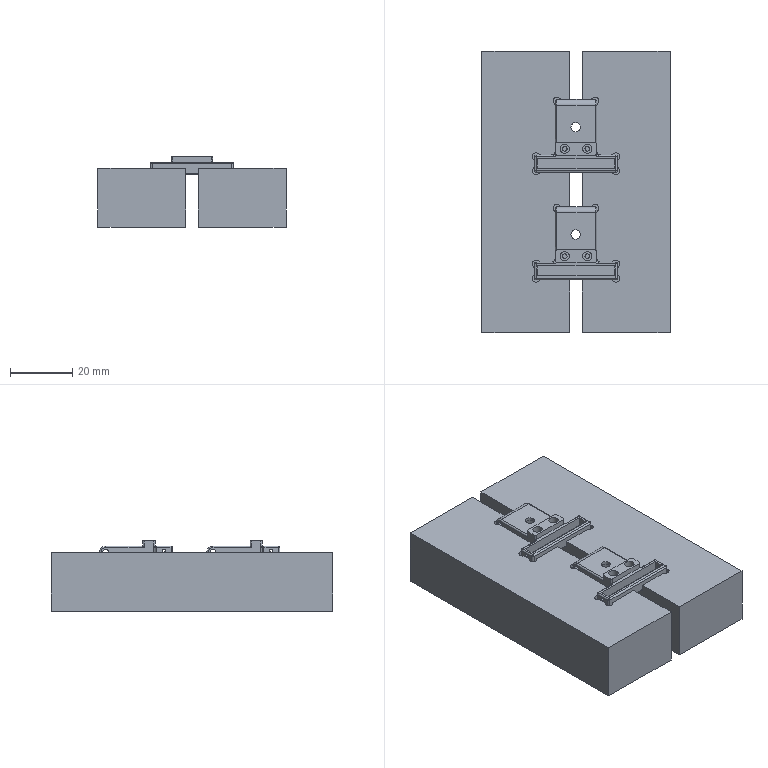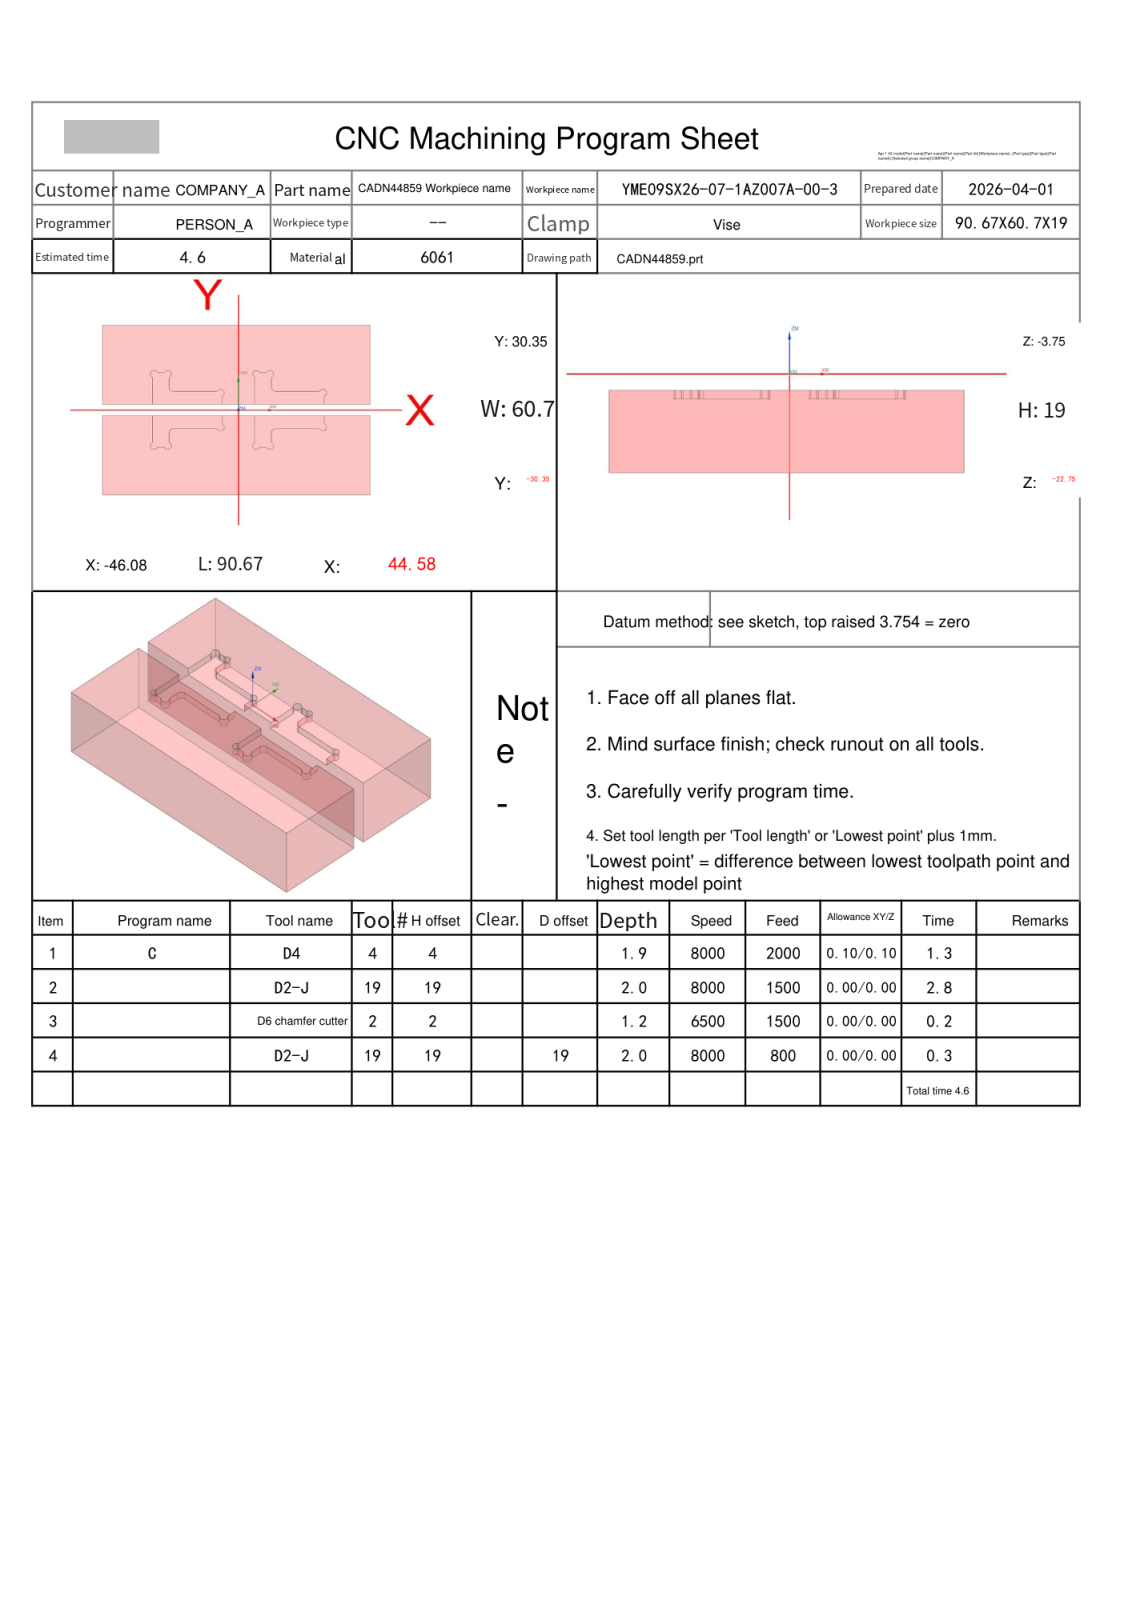NC program | NX | posted by the shop | part box 60.696 x 90.669 x 22.754 mm
Lines 950 to 1992 of 8014:
N2 T19 M06
(D2-J  D=2. R=0. H=19 ce=0.00 di=0.00)
G00 G90 G54 X27.884 Y3.83 M03 S8000
G43 H19 Z46.246
M08
Z-3.654
G01 X27.887 Z-3.684 F800.
X27.894 Y3.832 Z-3.712
X27.905 Y3.835 Z-3.736
X27.92 Y3.84 Z-3.758
X27.936 Y3.846 Z-3.777
X27.955 Y3.854 Z-3.794
X27.975 Y3.864 Z-3.808
X27.994 Y3.876 Z-3.82
X28.014 Y3.89 Z-3.83
X28.033 Y3.907 Z-3.838
X28.049 Y3.926 Z-3.844
X28.064 Y3.947 Z-3.849
X28.075 Y3.972 Z-3.852
X28.082 Y3.999 Z-3.853
X28.084 Y4.03 Z-3.854
Y4.698
G02 X28.727 Y5.929 I1.5 J0.0
G03 X28.834 Y6.134 I-.143 J.205
X28.584 Y6.384 I-.25 J0.0
X28.379 Y6.277 I0.0 J-.25
G02 X27.148 Y5.634 I-1.231 J.857
G01 X26.48
X26.454 Y5.62 Z-3.855
X26.45 Y5.582 Z-3.856
X26.465 Y5.524 Z-3.859
X26.497 Y5.448 Z-3.862
X26.544 Y5.359 Z-3.866
X26.602 Y5.26 Z-3.871
X26.671 Y5.156 Z-3.876
X26.747 Y5.049 Z-3.881
X26.974 Y4.772 Z-3.896
X27.229 Y4.516 Z-3.912
X27.504 Y4.289 Z-3.927
X27.61 Y4.214 Z-3.932
X27.714 Y4.146 Z-3.937
X27.811 Y4.089 Z-3.942
X27.9 Y4.043 Z-3.946
X27.975 Y4.013 Z-3.949
X28.033 Y3.999 Z-3.952
X28.071 Y4.003 Z-3.953
X28.084 Y4.03 Z-3.954
Y4.698
G02 X28.727 Y5.929 I1.5 J0.0
G03 X28.834 Y6.134 I-.143 J.205
X28.584 Y6.384 I-.25 J0.0
X28.379 Y6.277 I0.0 J-.25
G02 X27.148 Y5.634 I-1.231 J.857
G01 X26.48
X26.454 Y5.62 Z-3.955
X26.45 Y5.582 Z-3.956
X26.465 Y5.524 Z-3.959
X26.497 Y5.448 Z-3.962
X26.544 Y5.359 Z-3.966
X26.602 Y5.26 Z-3.971
X26.671 Y5.156 Z-3.976
X26.747 Y5.049 Z-3.981
X26.974 Y4.772 Z-3.996
X27.229 Y4.516 Z-4.012
X27.504 Y4.289 Z-4.027
X27.61 Y4.214 Z-4.032
X27.714 Y4.146 Z-4.037
X27.811 Y4.089 Z-4.042
X27.9 Y4.043 Z-4.046
X27.975 Y4.013 Z-4.049
X28.033 Y3.999 Z-4.052
X28.071 Y4.003 Z-4.053
X28.084 Y4.03 Z-4.054
Y4.698
G02 X28.727 Y5.929 I1.5 J0.0
G03 X28.834 Y6.134 I-.143 J.205
X28.584 Y6.384 I-.25 J0.0
X28.379 Y6.277 I0.0 J-.25
G02 X27.148 Y5.634 I-1.231 J.857
G01 X26.48
X26.454 Y5.62 Z-4.055
X26.45 Y5.582 Z-4.056
X26.465 Y5.524 Z-4.059
X26.497 Y5.448 Z-4.062
X26.544 Y5.359 Z-4.066
X26.602 Y5.26 Z-4.071
X26.671 Y5.156 Z-4.076
X26.747 Y5.049 Z-4.081
X26.974 Y4.772 Z-4.096
X27.229 Y4.516 Z-4.112
X27.504 Y4.289 Z-4.127
X27.61 Y4.214 Z-4.132
X27.714 Y4.146 Z-4.137
X27.811 Y4.089 Z-4.142
X27.9 Y4.043 Z-4.146
X27.975 Y4.013 Z-4.149
X28.033 Y3.999 Z-4.152
X28.071 Y4.003 Z-4.153
X28.084 Y4.03 Z-4.154
Y4.698
G02 X28.727 Y5.929 I1.5 J0.0
G03 X28.834 Y6.134 I-.143 J.205
X28.584 Y6.384 I-.25 J0.0
X28.379 Y6.277 I0.0 J-.25
G02 X27.148 Y5.634 I-1.231 J.857
G01 X26.48
X26.454 Y5.62 Z-4.155
X26.45 Y5.582 Z-4.156
X26.465 Y5.524 Z-4.159
X26.497 Y5.448 Z-4.162
X26.544 Y5.359 Z-4.166
X26.602 Y5.26 Z-4.171
X26.671 Y5.156 Z-4.176
X26.747 Y5.049 Z-4.181
X26.974 Y4.772 Z-4.196
X27.229 Y4.516 Z-4.212
X27.504 Y4.289 Z-4.227
X27.61 Y4.214 Z-4.232
X27.714 Y4.146 Z-4.237
X27.811 Y4.089 Z-4.242
X27.9 Y4.043 Z-4.246
X27.975 Y4.013 Z-4.249
X28.033 Y3.999 Z-4.252
X28.071 Y4.003 Z-4.253
X28.084 Y4.03 Z-4.254
Y4.698
G02 X28.727 Y5.929 I1.5 J0.0
G03 X28.834 Y6.134 I-.143 J.205
X28.584 Y6.384 I-.25 J0.0
X28.379 Y6.277 I0.0 J-.25
G02 X27.148 Y5.634 I-1.231 J.857
G01 X26.48
X26.454 Y5.62 Z-4.255
X26.45 Y5.582 Z-4.256
X26.465 Y5.524 Z-4.259
X26.497 Y5.448 Z-4.262
X26.544 Y5.359 Z-4.266
X26.602 Y5.26 Z-4.271
X26.671 Y5.156 Z-4.276
X26.747 Y5.049 Z-4.281
X26.974 Y4.772 Z-4.296
X27.229 Y4.516 Z-4.312
X27.504 Y4.289 Z-4.327
X27.61 Y4.214 Z-4.332
X27.714 Y4.146 Z-4.337
X27.811 Y4.089 Z-4.342
X27.9 Y4.043 Z-4.346
X27.975 Y4.013 Z-4.349
X28.033 Y3.999 Z-4.352
X28.071 Y4.003 Z-4.353
X28.084 Y4.03 Z-4.354
Y4.698
G02 X28.727 Y5.929 I1.5 J0.0
G03 X28.834 Y6.134 I-.143 J.205
X28.584 Y6.384 I-.25 J0.0
X28.379 Y6.277 I0.0 J-.25
G02 X27.148 Y5.634 I-1.231 J.857
G01 X26.48
X26.454 Y5.62 Z-4.355
X26.45 Y5.582 Z-4.356
X26.465 Y5.524 Z-4.359
X26.497 Y5.448 Z-4.362
X26.544 Y5.359 Z-4.366
X26.602 Y5.26 Z-4.371
X26.671 Y5.156 Z-4.376
X26.747 Y5.049 Z-4.381
X26.974 Y4.772 Z-4.396
X27.229 Y4.516 Z-4.412
X27.504 Y4.289 Z-4.427
X27.61 Y4.214 Z-4.432
X27.714 Y4.146 Z-4.437
X27.811 Y4.089 Z-4.442
X27.9 Y4.043 Z-4.446
X27.975 Y4.013 Z-4.449
X28.033 Y3.999 Z-4.452
X28.071 Y4.003 Z-4.453
X28.084 Y4.03 Z-4.454
Y4.698
G02 X28.727 Y5.929 I1.5 J0.0
G03 X28.834 Y6.134 I-.143 J.205
X28.584 Y6.384 I-.25 J0.0
X28.379 Y6.277 I0.0 J-.25
G02 X27.148 Y5.634 I-1.231 J.857
G01 X26.48
X26.454 Y5.62 Z-4.455
X26.45 Y5.582 Z-4.456
X26.465 Y5.524 Z-4.459
X26.497 Y5.448 Z-4.462
X26.544 Y5.359 Z-4.466
X26.602 Y5.26 Z-4.471
X26.671 Y5.156 Z-4.476
X26.747 Y5.049 Z-4.481
X26.974 Y4.772 Z-4.496
X27.229 Y4.516 Z-4.512
X27.504 Y4.289 Z-4.527
X27.61 Y4.214 Z-4.532
X27.714 Y4.146 Z-4.537
X27.811 Y4.089 Z-4.542
X27.9 Y4.043 Z-4.546
X27.975 Y4.013 Z-4.549
X28.033 Y3.999 Z-4.552
X28.071 Y4.003 Z-4.553
X28.084 Y4.03 Z-4.554
Y4.698
G02 X28.727 Y5.929 I1.5 J0.0
G03 X28.834 Y6.134 I-.143 J.205
X28.584 Y6.384 I-.25 J0.0
X28.379 Y6.277 I0.0 J-.25
G02 X27.148 Y5.634 I-1.231 J.857
G01 X26.48
X26.454 Y5.62 Z-4.555
X26.45 Y5.582 Z-4.556
X26.465 Y5.524 Z-4.559
X26.497 Y5.448 Z-4.562
X26.544 Y5.359 Z-4.566
X26.602 Y5.26 Z-4.571
X26.671 Y5.156 Z-4.576
X26.747 Y5.049 Z-4.581
X26.974 Y4.772 Z-4.596
X27.229 Y4.516 Z-4.612
X27.504 Y4.289 Z-4.627
X27.61 Y4.214 Z-4.632
X27.714 Y4.146 Z-4.637
X27.811 Y4.089 Z-4.642
X27.9 Y4.043 Z-4.646
X27.975 Y4.013 Z-4.649
X28.033 Y3.999 Z-4.652
X28.071 Y4.003 Z-4.653
X28.084 Y4.03 Z-4.654
Y4.698
G02 X28.727 Y5.929 I1.5 J0.0
G03 X28.834 Y6.134 I-.143 J.205
X28.584 Y6.384 I-.25 J0.0
X28.379 Y6.277 I0.0 J-.25
G02 X27.148 Y5.634 I-1.231 J.857
G01 X26.48
X26.454 Y5.62 Z-4.655
X26.45 Y5.582 Z-4.656
X26.465 Y5.524 Z-4.659
X26.497 Y5.448 Z-4.662
X26.544 Y5.359 Z-4.666
X26.602 Y5.26 Z-4.671
X26.671 Y5.156 Z-4.676
X26.747 Y5.049 Z-4.681
X26.974 Y4.772 Z-4.696
X27.229 Y4.516 Z-4.712
X27.504 Y4.289 Z-4.727
X27.61 Y4.214 Z-4.732
X27.714 Y4.146 Z-4.737
X27.811 Y4.089 Z-4.742
X27.9 Y4.043 Z-4.746
X27.975 Y4.013 Z-4.749
X28.033 Y3.999 Z-4.752
X28.071 Y4.003 Z-4.753
X28.084 Y4.03 Z-4.754
Y4.698
G02 X28.727 Y5.929 I1.5 J0.0
G03 X28.834 Y6.134 I-.143 J.205
X28.584 Y6.384 I-.25 J0.0
X28.379 Y6.277 I0.0 J-.25
G02 X27.148 Y5.634 I-1.231 J.857
G01 X26.48
X26.454 Y5.62 Z-4.755
X26.45 Y5.582 Z-4.756
X26.465 Y5.524 Z-4.759
X26.497 Y5.448 Z-4.762
X26.544 Y5.359 Z-4.766
X26.602 Y5.26 Z-4.771
X26.671 Y5.156 Z-4.776
X26.747 Y5.049 Z-4.781
X26.974 Y4.772 Z-4.796
X27.229 Y4.516 Z-4.812
X27.504 Y4.289 Z-4.827
X27.61 Y4.214 Z-4.832
X27.714 Y4.146 Z-4.837
X27.811 Y4.089 Z-4.842
X27.9 Y4.043 Z-4.846
X27.975 Y4.013 Z-4.849
X28.033 Y3.999 Z-4.852
X28.071 Y4.003 Z-4.853
X28.084 Y4.03 Z-4.854
Y4.698
G02 X28.727 Y5.929 I1.5 J0.0
G03 X28.834 Y6.134 I-.143 J.205
X28.584 Y6.384 I-.25 J0.0
X28.379 Y6.277 I0.0 J-.25
G02 X27.148 Y5.634 I-1.231 J.857
G01 X26.48
X26.454 Y5.62 Z-4.855
X26.45 Y5.582 Z-4.856
X26.465 Y5.524 Z-4.859
X26.497 Y5.448 Z-4.862
X26.544 Y5.359 Z-4.866
X26.602 Y5.26 Z-4.871
X26.671 Y5.156 Z-4.876
X26.747 Y5.049 Z-4.881
X26.974 Y4.772 Z-4.896
X27.229 Y4.516 Z-4.912
X27.504 Y4.289 Z-4.927
X27.61 Y4.214 Z-4.932
X27.714 Y4.146 Z-4.937
X27.811 Y4.089 Z-4.942
X27.9 Y4.043 Z-4.946
X27.975 Y4.013 Z-4.949
X28.033 Y3.999 Z-4.952
X28.071 Y4.003 Z-4.953
X28.084 Y4.03 Z-4.954
Y4.698
G02 X28.727 Y5.929 I1.5 J0.0
G03 X28.834 Y6.134 I-.143 J.205
X28.584 Y6.384 I-.25 J0.0
X28.379 Y6.277 I0.0 J-.25
G02 X27.148 Y5.634 I-1.231 J.857
G01 X26.48
X26.454 Y5.62 Z-4.955
X26.45 Y5.582 Z-4.956
X26.465 Y5.524 Z-4.959
X26.497 Y5.448 Z-4.962
X26.544 Y5.359 Z-4.966
X26.602 Y5.26 Z-4.971
X26.671 Y5.156 Z-4.976
X26.747 Y5.049 Z-4.981
X26.974 Y4.772 Z-4.996
X27.229 Y4.516 Z-5.012
X27.504 Y4.289 Z-5.027
X27.61 Y4.214 Z-5.032
X27.714 Y4.146 Z-5.037
X27.811 Y4.089 Z-5.042
X27.9 Y4.043 Z-5.046
X27.975 Y4.013 Z-5.049
X28.033 Y3.999 Z-5.052
X28.071 Y4.003 Z-5.053
X28.084 Y4.03 Z-5.054
Y4.698
G02 X28.727 Y5.929 I1.5 J0.0
G03 X28.834 Y6.134 I-.143 J.205
X28.584 Y6.384 I-.25 J0.0
X28.379 Y6.277 I0.0 J-.25
G02 X27.148 Y5.634 I-1.231 J.857
G01 X26.48
X26.454 Y5.62 Z-5.055
X26.45 Y5.582 Z-5.056
X26.465 Y5.524 Z-5.059
X26.497 Y5.448 Z-5.062
X26.544 Y5.359 Z-5.066
X26.602 Y5.26 Z-5.071
X26.671 Y5.156 Z-5.076
X26.747 Y5.049 Z-5.081
X26.974 Y4.772 Z-5.096
X27.229 Y4.516 Z-5.112
X27.504 Y4.289 Z-5.127
X27.61 Y4.214 Z-5.132
X27.714 Y4.146 Z-5.137
X27.811 Y4.089 Z-5.142
X27.9 Y4.043 Z-5.146
X27.975 Y4.013 Z-5.149
X28.033 Y3.999 Z-5.152
X28.071 Y4.003 Z-5.153
X28.084 Y4.03 Z-5.154
Y4.698
G02 X28.727 Y5.929 I1.5 J0.0
G03 X28.834 Y6.134 I-.143 J.205
X28.584 Y6.384 I-.25 J0.0
X28.379 Y6.277 I0.0 J-.25
G02 X27.148 Y5.634 I-1.231 J.857
G01 X26.48
X26.454 Y5.62 Z-5.155
X26.45 Y5.582 Z-5.156
X26.465 Y5.524 Z-5.159
X26.497 Y5.448 Z-5.162
X26.544 Y5.359 Z-5.166
X26.602 Y5.26 Z-5.171
X26.671 Y5.156 Z-5.176
X26.747 Y5.049 Z-5.181
X26.974 Y4.772 Z-5.196
X27.229 Y4.516 Z-5.212
X27.504 Y4.289 Z-5.227
X27.61 Y4.214 Z-5.232
X27.714 Y4.146 Z-5.237
X27.811 Y4.089 Z-5.242
X27.9 Y4.043 Z-5.246
X27.975 Y4.013 Z-5.249
X28.033 Y3.999 Z-5.252
X28.071 Y4.003 Z-5.253
X28.084 Y4.03 Z-5.254
Y4.698
G02 X28.727 Y5.929 I1.5 J0.0
G03 X28.834 Y6.134 I-.143 J.205
X28.584 Y6.384 I-.25 J0.0
X28.379 Y6.277 I0.0 J-.25
G02 X27.148 Y5.634 I-1.231 J.857
G01 X26.48
X26.454 Y5.62 Z-5.255
X26.45 Y5.582 Z-5.256
X26.465 Y5.524 Z-5.259
X26.497 Y5.448 Z-5.262
X26.544 Y5.359 Z-5.266
X26.602 Y5.26 Z-5.271
X26.671 Y5.156 Z-5.276
X26.747 Y5.049 Z-5.281
X26.974 Y4.772 Z-5.296
X27.229 Y4.516 Z-5.312
X27.504 Y4.289 Z-5.327
X27.61 Y4.214 Z-5.332
X27.714 Y4.146 Z-5.337
X27.811 Y4.089 Z-5.342
X27.9 Y4.043 Z-5.346
X27.975 Y4.013 Z-5.349
X28.033 Y3.999 Z-5.352
X28.071 Y4.003 Z-5.353
X28.084 Y4.03 Z-5.354
Y4.698
G02 X28.727 Y5.929 I1.5 J0.0
G03 X28.834 Y6.134 I-.143 J.205
X28.584 Y6.384 I-.25 J0.0
X28.379 Y6.277 I0.0 J-.25
G02 X27.148 Y5.634 I-1.231 J.857
G01 X26.48
X26.454 Y5.62 Z-5.355
X26.45 Y5.582 Z-5.356
X26.465 Y5.524 Z-5.359
X26.497 Y5.448 Z-5.362
X26.544 Y5.359 Z-5.366
X26.602 Y5.26 Z-5.371
X26.671 Y5.156 Z-5.376
X26.747 Y5.049 Z-5.381
X26.974 Y4.772 Z-5.396
X27.229 Y4.516 Z-5.412
X27.504 Y4.289 Z-5.427
X27.61 Y4.214 Z-5.432
X27.714 Y4.146 Z-5.437
X27.811 Y4.089 Z-5.442
X27.9 Y4.043 Z-5.446
X27.975 Y4.013 Z-5.449
X28.033 Y3.999 Z-5.452
X28.071 Y4.003 Z-5.453
X28.084 Y4.03 Z-5.454
Y4.698
G02 X28.727 Y5.929 I1.5 J0.0
G03 X28.834 Y6.134 I-.143 J.205
X28.584 Y6.384 I-.25 J0.0
X28.379 Y6.277 I0.0 J-.25
G02 X27.148 Y5.634 I-1.231 J.857
G01 X26.48
X26.454 Y5.62 Z-5.455
X26.45 Y5.582 Z-5.456
X26.465 Y5.524 Z-5.459
X26.497 Y5.448 Z-5.462
X26.544 Y5.359 Z-5.466
X26.602 Y5.26 Z-5.471
X26.671 Y5.156 Z-5.476
X26.747 Y5.049 Z-5.481
X26.974 Y4.772 Z-5.496
X27.229 Y4.516 Z-5.512
X27.504 Y4.289 Z-5.527
X27.61 Y4.214 Z-5.532
X27.714 Y4.146 Z-5.537
X27.811 Y4.089 Z-5.542
X27.9 Y4.043 Z-5.546
X27.975 Y4.013 Z-5.549
X28.033 Y3.999 Z-5.552
X28.071 Y4.003 Z-5.553
X28.084 Y4.03 Z-5.554
Y4.698
G02 X28.727 Y5.929 I1.5 J0.0
G03 X28.834 Y6.134 I-.143 J.205
X28.584 Y6.384 I-.25 J0.0
X28.379 Y6.277 I0.0 J-.25
G02 X27.148 Y5.634 I-1.231 J.857
G01 X26.48
X26.454 Y5.62 Z-5.555
X26.45 Y5.582 Z-5.556
X26.465 Y5.524 Z-5.559
X26.497 Y5.448 Z-5.562
X26.544 Y5.359 Z-5.566
X26.602 Y5.26 Z-5.571
X26.671 Y5.156 Z-5.576
X26.747 Y5.049 Z-5.581
X26.974 Y4.772 Z-5.596
X27.229 Y4.516 Z-5.612
X27.504 Y4.289 Z-5.627
X27.61 Y4.214 Z-5.632
X27.714 Y4.146 Z-5.637
X27.811 Y4.089 Z-5.642
X27.9 Y4.043 Z-5.646
X27.975 Y4.013 Z-5.649
X28.033 Y3.999 Z-5.652
X28.071 Y4.003 Z-5.653
X28.084 Y4.03 Z-5.654
Y4.698
G02 X28.727 Y5.929 I1.5 J0.0
G03 X28.834 Y6.134 I-.143 J.205
X28.584 Y6.384 I-.25 J0.0
X28.379 Y6.277 I0.0 J-.25
G02 X27.148 Y5.634 I-1.231 J.857
G01 X26.48
X26.454 Y5.62 Z-5.655
X26.45 Y5.582 Z-5.656
X26.465 Y5.524 Z-5.659
X26.497 Y5.448 Z-5.662
X26.544 Y5.359 Z-5.666
X26.602 Y5.26 Z-5.671
X26.671 Y5.156 Z-5.676
X26.747 Y5.049 Z-5.681
X26.974 Y4.772 Z-5.696
X27.229 Y4.516 Z-5.712
X27.504 Y4.289 Z-5.727
X27.61 Y4.214 Z-5.732
X27.714 Y4.146 Z-5.737
X27.811 Y4.089 Z-5.742
X27.9 Y4.043 Z-5.746
X27.975 Y4.013 Z-5.749
X28.033 Y3.999 Z-5.752
X28.071 Y4.003 Z-5.753
X28.084 Y4.03 Z-5.754
Y4.698
G02 X28.727 Y5.929 I1.5 J0.0
G03 X28.834 Y6.134 I-.143 J.205
X28.584 Y6.384 I-.25 J0.0
X28.379 Y6.277 I0.0 J-.25
G02 X27.148 Y5.634 I-1.231 J.857
G01 X26.48
X26.45 Y5.631 Z-5.753
X26.423 Y5.624 Z-5.752
X26.4 Y5.613 Z-5.749
X26.379 Y5.599 Z-5.744
X26.361 Y5.582 Z-5.738
X26.346 Y5.563 Z-5.73
X26.333 Y5.544 Z-5.72
X26.323 Y5.524 Z-5.708
X26.314 Y5.504 Z-5.694
X26.307 Y5.486 Z-5.677
X26.302 Y5.469 Z-5.658
X26.299 Y5.455 Z-5.636
X26.296 Y5.443 Z-5.612
X26.295 Y5.436 Z-5.584
Y5.434 Z-5.554
G00 Z46.246
X9.945 Y10.544
Z-3.654
G01 X9.947 Z-3.684
X9.955 Y10.546 Z-3.712
X9.966 Y10.549 Z-3.736
X9.98 Y10.554 Z-3.758
X9.997 Y10.56 Z-3.777
X10.016 Y10.568 Z-3.794
X10.036 Y10.578 Z-3.808
X10.056 Y10.59 Z-3.82
X10.076 Y10.604 Z-3.83
X10.095 Y10.621 Z-3.838
X10.112 Y10.64 Z-3.844
X10.127 Y10.662 Z-3.849
X10.138 Y10.686 Z-3.852
X10.145 Y10.713 Z-3.853
X10.148 Y10.744 Z-3.854
Y11.412
G02 X10.791 Y12.643 I1.5 J0.0
G03 X10.898 Y12.848 I-.143 J.205
X10.648 Y13.098 I-.25 J0.0
X10.443 Y12.991 I0.0 J-.25
G02 X9.212 Y12.348 I-1.231 J.857
G01 X8.543
X8.517 Y12.335 Z-3.855
X8.512 Y12.297 Z-3.856
X8.526 Y12.238 Z-3.859
X8.557 Y12.162 Z-3.862
X8.602 Y12.073 Z-3.866
X8.66 Y11.975 Z-3.871
X8.727 Y11.87 Z-3.876
X8.802 Y11.763 Z-3.881
X9.029 Y11.487 Z-3.896
X9.285 Y11.23 Z-3.912
X9.562 Y11.003 Z-3.927
X9.669 Y10.928 Z-3.932
X9.773 Y10.86 Z-3.937
X9.872 Y10.803 Z-3.942
X9.961 Y10.758 Z-3.946
X10.037 Y10.727 Z-3.949
X10.096 Y10.713 Z-3.952
X10.134 Y10.718 Z-3.953
X10.148 Y10.744 Z-3.954
Y11.412
G02 X10.791 Y12.643 I1.5 J0.0
G03 X10.898 Y12.848 I-.143 J.205
X10.648 Y13.098 I-.25 J0.0
X10.443 Y12.991 I0.0 J-.25
G02 X9.212 Y12.348 I-1.231 J.857
G01 X8.543
X8.517 Y12.335 Z-3.955
X8.512 Y12.297 Z-3.956
X8.526 Y12.238 Z-3.959
X8.557 Y12.162 Z-3.962
X8.602 Y12.073 Z-3.966
X8.66 Y11.975 Z-3.971
X8.727 Y11.87 Z-3.976
X8.802 Y11.763 Z-3.981
X9.029 Y11.487 Z-3.996
X9.285 Y11.23 Z-4.012
X9.562 Y11.003 Z-4.027
X9.669 Y10.928 Z-4.032
X9.773 Y10.86 Z-4.037
X9.872 Y10.803 Z-4.042
X9.961 Y10.758 Z-4.046
X10.037 Y10.727 Z-4.049
X10.096 Y10.713 Z-4.052
X10.134 Y10.718 Z-4.053
X10.148 Y10.744 Z-4.054
Y11.412
G02 X10.791 Y12.643 I1.5 J0.0
G03 X10.898 Y12.848 I-.143 J.205
X10.648 Y13.098 I-.25 J0.0
X10.443 Y12.991 I0.0 J-.25
G02 X9.212 Y12.348 I-1.231 J.857
G01 X8.543
X8.517 Y12.335 Z-4.055
X8.512 Y12.297 Z-4.056
X8.526 Y12.238 Z-4.059
X8.557 Y12.162 Z-4.062
X8.602 Y12.073 Z-4.066
X8.66 Y11.975 Z-4.071
X8.727 Y11.87 Z-4.076
X8.802 Y11.763 Z-4.081
X9.029 Y11.487 Z-4.096
X9.285 Y11.23 Z-4.112
X9.562 Y11.003 Z-4.127
X9.669 Y10.928 Z-4.132
X9.773 Y10.86 Z-4.137
X9.872 Y10.803 Z-4.142
X9.961 Y10.758 Z-4.146
X10.037 Y10.727 Z-4.149
X10.096 Y10.713 Z-4.152
X10.134 Y10.718 Z-4.153
X10.148 Y10.744 Z-4.154
Y11.412
G02 X10.791 Y12.643 I1.5 J0.0
G03 X10.898 Y12.848 I-.143 J.205
X10.648 Y13.098 I-.25 J0.0
X10.443 Y12.991 I0.0 J-.25
G02 X9.212 Y12.348 I-1.231 J.857
G01 X8.543
X8.517 Y12.335 Z-4.155
X8.512 Y12.297 Z-4.156
X8.526 Y12.238 Z-4.159
X8.557 Y12.162 Z-4.162
X8.602 Y12.073 Z-4.166
X8.66 Y11.975 Z-4.171
X8.727 Y11.87 Z-4.176
X8.802 Y11.763 Z-4.181
X9.029 Y11.487 Z-4.196
X9.285 Y11.23 Z-4.212
X9.562 Y11.003 Z-4.227
X9.669 Y10.928 Z-4.232
X9.773 Y10.86 Z-4.237
X9.872 Y10.803 Z-4.242
X9.961 Y10.758 Z-4.246
X10.037 Y10.727 Z-4.249
X10.096 Y10.713 Z-4.252
X10.134 Y10.718 Z-4.253
X10.148 Y10.744 Z-4.254
Y11.412
G02 X10.791 Y12.643 I1.5 J0.0
G03 X10.898 Y12.848 I-.143 J.205
X10.648 Y13.098 I-.25 J0.0
X10.443 Y12.991 I0.0 J-.25
G02 X9.212 Y12.348 I-1.231 J.857
G01 X8.543
X8.517 Y12.335 Z-4.255
X8.512 Y12.297 Z-4.256
X8.526 Y12.238 Z-4.259
X8.557 Y12.162 Z-4.262
X8.602 Y12.073 Z-4.266
X8.66 Y11.975 Z-4.271
X8.727 Y11.87 Z-4.276
X8.802 Y11.763 Z-4.281
X9.029 Y11.487 Z-4.296
X9.285 Y11.23 Z-4.312
X9.562 Y11.003 Z-4.327
X9.669 Y10.928 Z-4.332
X9.773 Y10.86 Z-4.337
X9.872 Y10.803 Z-4.342
X9.961 Y10.758 Z-4.346
X10.037 Y10.727 Z-4.349
X10.096 Y10.713 Z-4.352
X10.134 Y10.718 Z-4.353
X10.148 Y10.744 Z-4.354
Y11.412
G02 X10.791 Y12.643 I1.5 J0.0
G03 X10.898 Y12.848 I-.143 J.205
X10.648 Y13.098 I-.25 J0.0
X10.443 Y12.991 I0.0 J-.25
G02 X9.212 Y12.348 I-1.231 J.857
G01 X8.543
X8.517 Y12.335 Z-4.355
X8.512 Y12.297 Z-4.356
X8.526 Y12.238 Z-4.359
X8.557 Y12.162 Z-4.362
X8.602 Y12.073 Z-4.366
X8.66 Y11.975 Z-4.371
X8.727 Y11.87 Z-4.376
X8.802 Y11.763 Z-4.381
X9.029 Y11.487 Z-4.396
X9.285 Y11.23 Z-4.412
X9.562 Y11.003 Z-4.427
X9.669 Y10.928 Z-4.432
X9.773 Y10.86 Z-4.437
X9.872 Y10.803 Z-4.442
X9.961 Y10.758 Z-4.446
X10.037 Y10.727 Z-4.449
X10.096 Y10.713 Z-4.452
X10.134 Y10.718 Z-4.453
X10.148 Y10.744 Z-4.454
Y11.412
G02 X10.791 Y12.643 I1.5 J0.0
G03 X10.898 Y12.848 I-.143 J.205
X10.648 Y13.098 I-.25 J0.0
X10.443 Y12.991 I0.0 J-.25
G02 X9.212 Y12.348 I-1.231 J.857
G01 X8.543
X8.517 Y12.335 Z-4.455
X8.512 Y12.297 Z-4.456
X8.526 Y12.238 Z-4.459
X8.557 Y12.162 Z-4.462
X8.602 Y12.073 Z-4.466
X8.66 Y11.975 Z-4.471
X8.727 Y11.87 Z-4.476
X8.802 Y11.763 Z-4.481
X9.029 Y11.487 Z-4.496
X9.285 Y11.23 Z-4.512
X9.562 Y11.003 Z-4.527
X9.669 Y10.928 Z-4.532
X9.773 Y10.86 Z-4.537
X9.872 Y10.803 Z-4.542
X9.961 Y10.758 Z-4.546
X10.037 Y10.727 Z-4.549
X10.096 Y10.713 Z-4.552
X10.134 Y10.718 Z-4.553
X10.148 Y10.744 Z-4.554
Y11.412
G02 X10.791 Y12.643 I1.5 J0.0
G03 X10.898 Y12.848 I-.143 J.205
X10.648 Y13.098 I-.25 J0.0
X10.443 Y12.991 I0.0 J-.25
G02 X9.212 Y12.348 I-1.231 J.857
G01 X8.543
X8.517 Y12.335 Z-4.555
X8.512 Y12.297 Z-4.556
X8.526 Y12.238 Z-4.559
X8.557 Y12.162 Z-4.562
X8.602 Y12.073 Z-4.566
X8.66 Y11.975 Z-4.571
X8.727 Y11.87 Z-4.576
X8.802 Y11.763 Z-4.581
X9.029 Y11.487 Z-4.596
X9.285 Y11.23 Z-4.612
X9.562 Y11.003 Z-4.627
X9.669 Y10.928 Z-4.632
X9.773 Y10.86 Z-4.637
X9.872 Y10.803 Z-4.642
X9.961 Y10.758 Z-4.646
X10.037 Y10.727 Z-4.649
X10.096 Y10.713 Z-4.652
X10.134 Y10.718 Z-4.653
X10.148 Y10.744 Z-4.654
Y11.412
G02 X10.791 Y12.643 I1.5 J0.0
G03 X10.898 Y12.848 I-.143 J.205
X10.648 Y13.098 I-.25 J0.0
X10.443 Y12.991 I0.0 J-.25
G02 X9.212 Y12.348 I-1.231 J.857
G01 X8.543
X8.517 Y12.335 Z-4.655
X8.512 Y12.297 Z-4.656
X8.526 Y12.238 Z-4.659
X8.557 Y12.162 Z-4.662
X8.602 Y12.073 Z-4.666
X8.66 Y11.975 Z-4.671
X8.727 Y11.87 Z-4.676
X8.802 Y11.763 Z-4.681
X9.029 Y11.487 Z-4.696
X9.285 Y11.23 Z-4.712
X9.562 Y11.003 Z-4.727
X9.669 Y10.928 Z-4.732
X9.773 Y10.86 Z-4.737
X9.872 Y10.803 Z-4.742
X9.961 Y10.758 Z-4.746
X10.037 Y10.727 Z-4.749
X10.096 Y10.713 Z-4.752
X10.134 Y10.718 Z-4.753
X10.148 Y10.744 Z-4.754
Y11.412
G02 X10.791 Y12.643 I1.5 J0.0
G03 X10.898 Y12.848 I-.143 J.205
X10.648 Y13.098 I-.25 J0.0
X10.443 Y12.991 I0.0 J-.25
G02 X9.212 Y12.348 I-1.231 J.857
G01 X8.543
X8.517 Y12.335 Z-4.755
X8.512 Y12.297 Z-4.756
X8.526 Y12.238 Z-4.759
X8.557 Y12.162 Z-4.762
X8.602 Y12.073 Z-4.766
X8.66 Y11.975 Z-4.771
X8.727 Y11.87 Z-4.776
X8.802 Y11.763 Z-4.781
X9.029 Y11.487 Z-4.796
X9.285 Y11.23 Z-4.812
X9.562 Y11.003 Z-4.827
X9.669 Y10.928 Z-4.832
X9.773 Y10.86 Z-4.837
X9.872 Y10.803 Z-4.842
X9.961 Y10.758 Z-4.846
X10.037 Y10.727 Z-4.849
X10.096 Y10.713 Z-4.852
X10.134 Y10.718 Z-4.853
X10.148 Y10.744 Z-4.854
Y11.412
G02 X10.791 Y12.643 I1.5 J0.0
G03 X10.898 Y12.848 I-.143 J.205
X10.648 Y13.098 I-.25 J0.0
X10.443 Y12.991 I0.0 J-.25
G02 X9.212 Y12.348 I-1.231 J.857
G01 X8.543
X8.517 Y12.335 Z-4.855
X8.512 Y12.297 Z-4.856
X8.526 Y12.238 Z-4.859
X8.557 Y12.162 Z-4.862
X8.602 Y12.073 Z-4.866
X8.66 Y11.975 Z-4.871
X8.727 Y11.87 Z-4.876
X8.802 Y11.763 Z-4.881
X9.029 Y11.487 Z-4.896
X9.285 Y11.23 Z-4.912
X9.562 Y11.003 Z-4.927
X9.669 Y10.928 Z-4.932
X9.773 Y10.86 Z-4.937
X9.872 Y10.803 Z-4.942
X9.961 Y10.758 Z-4.946
X10.037 Y10.727 Z-4.949
X10.096 Y10.713 Z-4.952
X10.134 Y10.718 Z-4.953
X10.148 Y10.744 Z-4.954
Y11.412
G02 X10.791 Y12.643 I1.5 J0.0
G03 X10.898 Y12.848 I-.143 J.205
X10.648 Y13.098 I-.25 J0.0
X10.443 Y12.991 I0.0 J-.25
G02 X9.212 Y12.348 I-1.231 J.857
G01 X8.543
X8.517 Y12.335 Z-4.955
X8.512 Y12.297 Z-4.956
X8.526 Y12.238 Z-4.959
X8.557 Y12.162 Z-4.962
X8.602 Y12.073 Z-4.966
X8.66 Y11.975 Z-4.971
X8.727 Y11.87 Z-4.976
X8.802 Y11.763 Z-4.981
X9.029 Y11.487 Z-4.996
X9.285 Y11.23 Z-5.012
X9.562 Y11.003 Z-5.027
X9.669 Y10.928 Z-5.032
X9.773 Y10.86 Z-5.037
X9.872 Y10.803 Z-5.042
X9.961 Y10.758 Z-5.046
X10.037 Y10.727 Z-5.049
X10.096 Y10.713 Z-5.052
X10.134 Y10.718 Z-5.053
X10.148 Y10.744 Z-5.054
Y11.412
G02 X10.791 Y12.643 I1.5 J0.0
G03 X10.898 Y12.848 I-.143 J.205
X10.648 Y13.098 I-.25 J0.0
X10.443 Y12.991 I0.0 J-.25
G02 X9.212 Y12.348 I-1.231 J.857
G01 X8.543
X8.517 Y12.335 Z-5.055
X8.512 Y12.297 Z-5.056
X8.526 Y12.238 Z-5.059
X8.557 Y12.162 Z-5.062
X8.602 Y12.073 Z-5.066
X8.66 Y11.975 Z-5.071
X8.727 Y11.87 Z-5.076
X8.802 Y11.763 Z-5.081
X9.029 Y11.487 Z-5.096
X9.285 Y11.23 Z-5.112
X9.562 Y11.003 Z-5.127
X9.669 Y10.928 Z-5.132
X9.773 Y10.86 Z-5.137
X9.872 Y10.803 Z-5.142
X9.961 Y10.758 Z-5.146
X10.037 Y10.727 Z-5.149
X10.096 Y10.713 Z-5.152
X10.134 Y10.718 Z-5.153
X10.148 Y10.744 Z-5.154
Y11.412
G02 X10.791 Y12.643 I1.5 J0.0
G03 X10.898 Y12.848 I-.143 J.205
X10.648 Y13.098 I-.25 J0.0
X10.443 Y12.991 I0.0 J-.25
G02 X9.212 Y12.348 I-1.231 J.857
G01 X8.543
X8.517 Y12.335 Z-5.155
X8.512 Y12.297 Z-5.156
X8.526 Y12.238 Z-5.159
X8.557 Y12.162 Z-5.162
X8.602 Y12.073 Z-5.166
X8.66 Y11.975 Z-5.171
X8.727 Y11.87 Z-5.176
X8.802 Y11.763 Z-5.181
X9.029 Y11.487 Z-5.196
X9.285 Y11.23 Z-5.212
X9.562 Y11.003 Z-5.227
X9.669 Y10.928 Z-5.232
X9.773 Y10.86 Z-5.237
X9.872 Y10.803 Z-5.242
X9.961 Y10.758 Z-5.246
X10.037 Y10.727 Z-5.249
X10.096 Y10.713 Z-5.252
X10.134 Y10.718 Z-5.253
X10.148 Y10.744 Z-5.254
Y11.412
G02 X10.791 Y12.643 I1.5 J0.0
G03 X10.898 Y12.848 I-.143 J.205
X10.648 Y13.098 I-.25 J0.0
X10.443 Y12.991 I0.0 J-.25
G02 X9.212 Y12.348 I-1.231 J.857
G01 X8.543
X8.517 Y12.335 Z-5.255
X8.512 Y12.297 Z-5.256
X8.526 Y12.238 Z-5.259
X8.557 Y12.162 Z-5.262
X8.602 Y12.073 Z-5.266
X8.66 Y11.975 Z-5.271
X8.727 Y11.87 Z-5.276
X8.802 Y11.763 Z-5.281
X9.029 Y11.487 Z-5.296
X9.285 Y11.23 Z-5.312
X9.562 Y11.003 Z-5.327
X9.669 Y10.928 Z-5.332
X9.773 Y10.86 Z-5.337
X9.872 Y10.803 Z-5.342
X9.961 Y10.758 Z-5.346
X10.037 Y10.727 Z-5.349
X10.096 Y10.713 Z-5.352
X10.134 Y10.718 Z-5.353
X10.148 Y10.744 Z-5.354
Y11.412
G02 X10.791 Y12.643 I1.5 J0.0
G03 X10.898 Y12.848 I-.143 J.205
X10.648 Y13.098 I-.25 J0.0
X10.443 Y12.991 I0.0 J-.25
G02 X9.212 Y12.348 I-1.231 J.857
G01 X8.543
X8.517 Y12.335 Z-5.355
X8.512 Y12.297 Z-5.356
X8.526 Y12.238 Z-5.359
X8.557 Y12.162 Z-5.362
X8.602 Y12.073 Z-5.366
X8.66 Y11.975 Z-5.371
X8.727 Y11.87 Z-5.376
X8.802 Y11.763 Z-5.381
X9.029 Y11.487 Z-5.396
X9.285 Y11.23 Z-5.412
X9.562 Y11.003 Z-5.427
X9.669 Y10.928 Z-5.432
X9.773 Y10.86 Z-5.437
X9.872 Y10.803 Z-5.442
X9.961 Y10.758 Z-5.446
X10.037 Y10.727 Z-5.449
X10.096 Y10.713 Z-5.452
X10.134 Y10.718 Z-5.453
X10.148 Y10.744 Z-5.454
Y11.412
G02 X10.791 Y12.643 I1.5 J0.0
G03 X10.898 Y12.848 I-.143 J.205
X10.648 Y13.098 I-.25 J0.0
X10.443 Y12.991 I0.0 J-.25
G02 X9.212 Y12.348 I-1.231 J.857
G01 X8.543
X8.517 Y12.335 Z-5.455
X8.512 Y12.297 Z-5.456
X8.526 Y12.238 Z-5.459
X8.557 Y12.162 Z-5.462
X8.602 Y12.073 Z-5.466
X8.66 Y11.975 Z-5.471
X8.727 Y11.87 Z-5.476
X8.802 Y11.763 Z-5.481
X9.029 Y11.487 Z-5.496
X9.285 Y11.23 Z-5.512
X9.562 Y11.003 Z-5.527
X9.669 Y10.928 Z-5.532
X9.773 Y10.86 Z-5.537
X9.872 Y10.803 Z-5.542
X9.961 Y10.758 Z-5.546
X10.037 Y10.727 Z-5.549
X10.096 Y10.713 Z-5.552
X10.134 Y10.718 Z-5.553
X10.148 Y10.744 Z-5.554
Y11.412
G02 X10.791 Y12.643 I1.5 J0.0
G03 X10.898 Y12.848 I-.143 J.205
X10.648 Y13.098 I-.25 J0.0
X10.443 Y12.991 I0.0 J-.25
G02 X9.212 Y12.348 I-1.231 J.857
G01 X8.543
X8.517 Y12.335 Z-5.555
X8.512 Y12.297 Z-5.556
X8.526 Y12.238 Z-5.559
X8.557 Y12.162 Z-5.562
X8.602 Y12.073 Z-5.566
X8.66 Y11.975 Z-5.571
X8.727 Y11.87 Z-5.576
X8.802 Y11.763 Z-5.581
X9.029 Y11.487 Z-5.596
X9.285 Y11.23 Z-5.612
X9.562 Y11.003 Z-5.627
X9.669 Y10.928 Z-5.632
X9.773 Y10.86 Z-5.637
X9.872 Y10.803 Z-5.642
X9.961 Y10.758 Z-5.646
X10.037 Y10.727 Z-5.649
X10.096 Y10.713 Z-5.652
X10.134 Y10.718 Z-5.653
X10.148 Y10.744 Z-5.654
Y11.412
G02 X10.791 Y12.643 I1.5 J0.0
G03 X10.898 Y12.848 I-.143 J.205
X10.648 Y13.098 I-.25 J0.0
X10.443 Y12.991 I0.0 J-.25
G02 X9.212 Y12.348 I-1.231 J.857
G01 X8.543
X8.517 Y12.335 Z-5.655
X8.512 Y12.297 Z-5.656
X8.526 Y12.238 Z-5.659
X8.557 Y12.162 Z-5.662
X8.602 Y12.073 Z-5.666
X8.66 Y11.975 Z-5.671
X8.727 Y11.87 Z-5.676
X8.802 Y11.763 Z-5.681
X9.029 Y11.487 Z-5.696
X9.285 Y11.23 Z-5.712
X9.562 Y11.003 Z-5.727
X9.669 Y10.928 Z-5.732
X9.773 Y10.86 Z-5.737